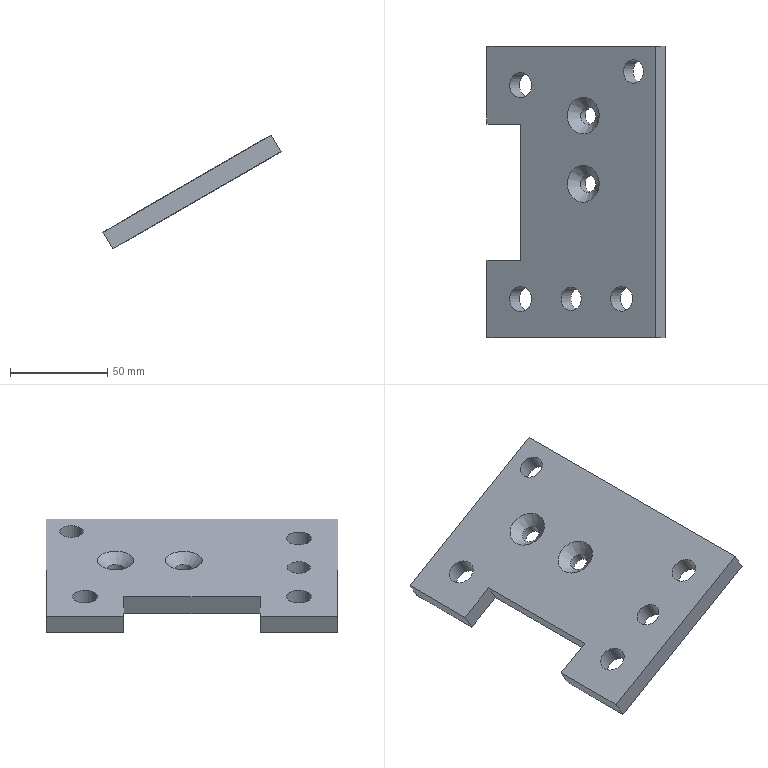Part | NX | features solid 2 | 1 solid | 19 faces | box 91.603 x 150 x 58.66 mm | volume 127515 mm3 | plane 10 | cylinder 7 | cone 2 | commonest cylinder face diameters 13 x3 9 x2 12 x2
STEP:
#1=CARTESIAN_POINT('',(89.575,759.782,201.044));
#2=VERTEX_POINT('',#1);
#3=CARTESIAN_POINT('',(89.575,764.282,201.044));
#4=DIRECTION('',(-0.5,0.,0.866));
#5=DIRECTION('',(0.,-1.,0.));
#6=AXIS2_PLACEMENT_3D('',#3,#4,#5);
#7=CIRCLE('',#6,4.5);
#8=EDGE_CURVE('',#2,#2,#7,.T.);
#9=ORIENTED_EDGE('',*,*,#8,.T.);
#10=EDGE_LOOP('',(#9));
#11=FACE_BOUND('',#10,.T.);
#12=CARTESIAN_POINT('',(120.538,787.,218.92));
#13=VERTEX_POINT('',#12);
#14=CARTESIAN_POINT('',(115.342,787.,215.92));
#15=DIRECTION('',(-0.5,0.,0.866));
#16=DIRECTION('',(0.866,0.,0.5));
#17=AXIS2_PLACEMENT_3D('',#14,#15,#16);
#18=CIRCLE('',#17,6.);
#19=EDGE_CURVE('',#13,#13,#18,.T.);
#20=ORIENTED_EDGE('',*,*,#19,.T.);
#21=EDGE_LOOP('',(#20));
#22=FACE_BOUND('',#21,.T.);
#23=CARTESIAN_POINT('',(62.947,670.,185.67));
#24=VERTEX_POINT('',#23);
#25=CARTESIAN_POINT('',(57.318,670.,182.42));
#26=DIRECTION('',(-0.5,0.,0.866));
#27=DIRECTION('',(0.866,0.,0.5));
#28=AXIS2_PLACEMENT_3D('',#25,#26,#27);
#29=CIRCLE('',#28,6.5);
#30=EDGE_CURVE('',#24,#24,#29,.T.);
#31=ORIENTED_EDGE('',*,*,#30,.T.);
#32=EDGE_LOOP('',(#31));
#33=FACE_BOUND('',#32,.T.);
#34=CARTESIAN_POINT('',(39.997,650.,172.42));
#35=VERTEX_POINT('',#34);
#36=CARTESIAN_POINT('',(39.997,690.,172.42));
#37=VERTEX_POINT('',#36);
#38=CARTESIAN_POINT('',(39.997,650.,172.42));
#39=DIRECTION('',(0.,-1.,0.));
#40=VECTOR('',#39,1000.);
#41=LINE('',#38,#40);
#42=EDGE_CURVE('',#35,#37,#41,.F.);
#43=ORIENTED_EDGE('',*,*,#42,.T.);
#44=CARTESIAN_POINT('',(57.318,690.,182.42));
#45=VERTEX_POINT('',#44);
#46=CARTESIAN_POINT('',(111.6,690.,213.759));
#47=DIRECTION('',(-0.866,0.,-0.5));
#48=VECTOR('',#47,1000.);
#49=LINE('',#46,#48);
#50=EDGE_CURVE('',#37,#45,#49,.F.);
#51=ORIENTED_EDGE('',*,*,#50,.T.);
#52=CARTESIAN_POINT('',(57.318,760.,182.42));
#53=VERTEX_POINT('',#52);
#54=CARTESIAN_POINT('',(57.318,650.,182.42));
#55=DIRECTION('',(0.,-1.,0.));
#56=VECTOR('',#55,1000.);
#57=LINE('',#54,#56);
#58=EDGE_CURVE('',#45,#53,#57,.F.);
#59=ORIENTED_EDGE('',*,*,#58,.T.);
#60=CARTESIAN_POINT('',(39.997,760.,172.42));
#61=VERTEX_POINT('',#60);
#62=CARTESIAN_POINT('',(24.997,760.,163.759));
#63=DIRECTION('',(0.866,0.,0.5));
#64=VECTOR('',#63,1000.);
#65=LINE('',#62,#64);
#66=EDGE_CURVE('',#61,#53,#65,.T.);
#67=ORIENTED_EDGE('',*,*,#66,.F.);
#68=CARTESIAN_POINT('',(39.997,800.,172.42));
#69=VERTEX_POINT('',#68);
#70=CARTESIAN_POINT('',(39.997,650.,172.42));
#71=DIRECTION('',(0.,-1.,0.));
#72=VECTOR('',#71,1000.);
#73=LINE('',#70,#72);
#74=EDGE_CURVE('',#61,#69,#73,.F.);
#75=ORIENTED_EDGE('',*,*,#74,.T.);
#76=CARTESIAN_POINT('',(126.6,800.,222.42));
#77=VERTEX_POINT('',#76);
#78=CARTESIAN_POINT('',(111.6,800.,213.759));
#79=DIRECTION('',(-0.866,0.,-0.5));
#80=VECTOR('',#79,1000.);
#81=LINE('',#78,#80);
#82=EDGE_CURVE('',#77,#69,#81,.T.);
#83=ORIENTED_EDGE('',*,*,#82,.F.);
#84=CARTESIAN_POINT('',(126.6,650.,222.42));
#85=VERTEX_POINT('',#84);
#86=CARTESIAN_POINT('',(126.6,650.,222.42));
#87=DIRECTION('',(0.,1.,0.));
#88=VECTOR('',#87,1000.);
#89=LINE('',#86,#88);
#90=EDGE_CURVE('',#85,#77,#89,.T.);
#91=ORIENTED_EDGE('',*,*,#90,.F.);
#92=CARTESIAN_POINT('',(111.6,650.,213.759));
#93=DIRECTION('',(0.866,0.,0.5));
#94=VECTOR('',#93,1000.);
#95=LINE('',#92,#94);
#96=EDGE_CURVE('',#85,#35,#95,.F.);
#97=ORIENTED_EDGE('',*,*,#96,.T.);
#98=EDGE_LOOP('',(#43,#51,#59,#67,#75,#83,#91,#97));
#99=FACE_BOUND('',#98,.T.);
#100=CARTESIAN_POINT('',(62.947,780.,185.67));
#101=VERTEX_POINT('',#100);
#102=CARTESIAN_POINT('',(57.318,780.,182.42));
#103=DIRECTION('',(-0.5,0.,0.866));
#104=DIRECTION('',(0.866,0.,0.5));
#105=AXIS2_PLACEMENT_3D('',#102,#103,#104);
#106=CIRCLE('',#105,6.5);
#107=EDGE_CURVE('',#101,#101,#106,.T.);
#108=ORIENTED_EDGE('',*,*,#107,.T.);
#109=EDGE_LOOP('',(#108));
#110=FACE_BOUND('',#109,.T.);
#111=CARTESIAN_POINT('',(114.909,670.,215.67));
#112=VERTEX_POINT('',#111);
#113=CARTESIAN_POINT('',(109.279,670.,212.42));
#114=DIRECTION('',(-0.5,0.,0.866));
#115=DIRECTION('',(0.866,0.,0.5));
#116=AXIS2_PLACEMENT_3D('',#113,#114,#115);
#117=CIRCLE('',#116,6.5);
#118=EDGE_CURVE('',#112,#112,#117,.T.);
#119=ORIENTED_EDGE('',*,*,#118,.T.);
#120=EDGE_LOOP('',(#119));
#121=FACE_BOUND('',#120,.T.);
#122=CARTESIAN_POINT('',(88.495,670.,200.42));
#123=VERTEX_POINT('',#122);
#124=CARTESIAN_POINT('',(83.299,670.,197.42));
#125=DIRECTION('',(-0.5,0.,0.866));
#126=DIRECTION('',(0.866,0.,0.5));
#127=AXIS2_PLACEMENT_3D('',#124,#125,#126);
#128=CIRCLE('',#127,6.);
#129=EDGE_CURVE('',#123,#123,#128,.T.);
#130=ORIENTED_EDGE('',*,*,#129,.T.);
#131=EDGE_LOOP('',(#130));
#132=FACE_BOUND('',#131,.T.);
#133=CARTESIAN_POINT('',(89.542,724.74,201.024));
#134=VERTEX_POINT('',#133);
#135=CARTESIAN_POINT('',(89.542,729.24,201.024));
#136=DIRECTION('',(-0.5,0.,0.866));
#137=DIRECTION('',(0.,-1.,0.));
#138=AXIS2_PLACEMENT_3D('',#135,#136,#137);
#139=CIRCLE('',#138,4.5);
#140=EDGE_CURVE('',#134,#134,#139,.T.);
#141=ORIENTED_EDGE('',*,*,#140,.T.);
#142=EDGE_LOOP('',(#141));
#143=FACE_BOUND('',#142,.T.);
#144=CARTESIAN_POINT('',(111.6,650.,213.759));
#145=DIRECTION('',(-0.5,0.,0.866));
#146=DIRECTION('',(-0.866,0.,-0.5));
#147=AXIS2_PLACEMENT_3D('',#144,#145,#146);
#148=PLANE('',#147);
#149=ADVANCED_FACE('',(#11,#22,#33,#99,#110,#121,#132,#143),#148,.F.);
#150=CARTESIAN_POINT('',(92.803,764.282,214.454));
#151=VERTEX_POINT('',#150);
#152=CARTESIAN_POINT('',(84.575,764.282,209.704));
#153=DIRECTION('',(-0.5,0.,0.866));
#154=DIRECTION('',(0.866,0.,0.5));
#155=AXIS2_PLACEMENT_3D('',#152,#153,#154);
#156=CIRCLE('',#155,9.5);
#157=EDGE_CURVE('',#151,#151,#156,.T.);
#158=ORIENTED_EDGE('',*,*,#157,.F.);
#159=EDGE_LOOP('',(#158));
#160=FACE_BOUND('',#159,.T.);
#161=CARTESIAN_POINT('',(92.769,729.24,214.434));
#162=VERTEX_POINT('',#161);
#163=CARTESIAN_POINT('',(84.542,729.24,209.684));
#164=DIRECTION('',(-0.5,0.,0.866));
#165=DIRECTION('',(0.866,0.,0.5));
#166=AXIS2_PLACEMENT_3D('',#163,#164,#165);
#167=CIRCLE('',#166,9.5);
#168=EDGE_CURVE('',#162,#162,#167,.T.);
#169=ORIENTED_EDGE('',*,*,#168,.F.);
#170=EDGE_LOOP('',(#169));
#171=FACE_BOUND('',#170,.T.);
#172=CARTESIAN_POINT('',(115.538,787.,227.58));
#173=VERTEX_POINT('',#172);
#174=CARTESIAN_POINT('',(110.342,787.,224.58));
#175=DIRECTION('',(-0.5,0.,0.866));
#176=DIRECTION('',(0.866,0.,0.5));
#177=AXIS2_PLACEMENT_3D('',#174,#175,#176);
#178=CIRCLE('',#177,6.);
#179=EDGE_CURVE('',#173,#173,#178,.T.);
#180=ORIENTED_EDGE('',*,*,#179,.F.);
#181=EDGE_LOOP('',(#180));
#182=FACE_BOUND('',#181,.T.);
#183=CARTESIAN_POINT('',(57.947,670.,194.33));
#184=VERTEX_POINT('',#183);
#185=CARTESIAN_POINT('',(52.318,670.,191.08));
#186=DIRECTION('',(-0.5,0.,0.866));
#187=DIRECTION('',(0.866,0.,0.5));
#188=AXIS2_PLACEMENT_3D('',#185,#186,#187);
#189=CIRCLE('',#188,6.5);
#190=EDGE_CURVE('',#184,#184,#189,.T.);
#191=ORIENTED_EDGE('',*,*,#190,.F.);
#192=EDGE_LOOP('',(#191));
#193=FACE_BOUND('',#192,.T.);
#194=CARTESIAN_POINT('',(34.997,690.,181.08));
#195=VERTEX_POINT('',#194);
#196=CARTESIAN_POINT('',(52.318,690.,191.08));
#197=VERTEX_POINT('',#196);
#198=CARTESIAN_POINT('',(19.997,690.,172.42));
#199=DIRECTION('',(-0.866,0.,-0.5));
#200=VECTOR('',#199,1000.);
#201=LINE('',#198,#200);
#202=EDGE_CURVE('',#195,#197,#201,.F.);
#203=ORIENTED_EDGE('',*,*,#202,.F.);
#204=CARTESIAN_POINT('',(34.997,650.,181.08));
#205=VERTEX_POINT('',#204);
#206=CARTESIAN_POINT('',(34.997,650.,181.08));
#207=DIRECTION('',(0.,-1.,0.));
#208=VECTOR('',#207,1000.);
#209=LINE('',#206,#208);
#210=EDGE_CURVE('',#205,#195,#209,.F.);
#211=ORIENTED_EDGE('',*,*,#210,.F.);
#212=CARTESIAN_POINT('',(121.6,650.,231.08));
#213=VERTEX_POINT('',#212);
#214=CARTESIAN_POINT('',(106.6,650.,222.42));
#215=DIRECTION('',(-0.866,0.,-0.5));
#216=VECTOR('',#215,1000.);
#217=LINE('',#214,#216);
#218=EDGE_CURVE('',#213,#205,#217,.T.);
#219=ORIENTED_EDGE('',*,*,#218,.F.);
#220=CARTESIAN_POINT('',(121.6,800.,231.08));
#221=VERTEX_POINT('',#220);
#222=CARTESIAN_POINT('',(121.6,650.,231.08));
#223=DIRECTION('',(0.,1.,0.));
#224=VECTOR('',#223,1000.);
#225=LINE('',#222,#224);
#226=EDGE_CURVE('',#213,#221,#225,.T.);
#227=ORIENTED_EDGE('',*,*,#226,.T.);
#228=CARTESIAN_POINT('',(34.997,800.,181.08));
#229=VERTEX_POINT('',#228);
#230=CARTESIAN_POINT('',(106.6,800.,222.42));
#231=DIRECTION('',(-0.866,0.,-0.5));
#232=VECTOR('',#231,1000.);
#233=LINE('',#230,#232);
#234=EDGE_CURVE('',#221,#229,#233,.T.);
#235=ORIENTED_EDGE('',*,*,#234,.T.);
#236=CARTESIAN_POINT('',(34.997,760.,181.08));
#237=VERTEX_POINT('',#236);
#238=CARTESIAN_POINT('',(34.997,650.,181.08));
#239=DIRECTION('',(0.,-1.,0.));
#240=VECTOR('',#239,1000.);
#241=LINE('',#238,#240);
#242=EDGE_CURVE('',#237,#229,#241,.F.);
#243=ORIENTED_EDGE('',*,*,#242,.F.);
#244=CARTESIAN_POINT('',(52.318,760.,191.08));
#245=VERTEX_POINT('',#244);
#246=CARTESIAN_POINT('',(19.997,760.,172.42));
#247=DIRECTION('',(0.866,0.,0.5));
#248=VECTOR('',#247,1000.);
#249=LINE('',#246,#248);
#250=EDGE_CURVE('',#237,#245,#249,.T.);
#251=ORIENTED_EDGE('',*,*,#250,.T.);
#252=CARTESIAN_POINT('',(52.318,650.,191.08));
#253=DIRECTION('',(0.,-1.,0.));
#254=VECTOR('',#253,1000.);
#255=LINE('',#252,#254);
#256=EDGE_CURVE('',#197,#245,#255,.F.);
#257=ORIENTED_EDGE('',*,*,#256,.F.);
#258=EDGE_LOOP('',(#203,#211,#219,#227,#235,#243,#251,#257));
#259=FACE_BOUND('',#258,.T.);
#260=CARTESIAN_POINT('',(57.947,780.,194.33));
#261=VERTEX_POINT('',#260);
#262=CARTESIAN_POINT('',(52.318,780.,191.08));
#263=DIRECTION('',(-0.5,0.,0.866));
#264=DIRECTION('',(0.866,0.,0.5));
#265=AXIS2_PLACEMENT_3D('',#262,#263,#264);
#266=CIRCLE('',#265,6.5);
#267=EDGE_CURVE('',#261,#261,#266,.T.);
#268=ORIENTED_EDGE('',*,*,#267,.F.);
#269=EDGE_LOOP('',(#268));
#270=FACE_BOUND('',#269,.T.);
#271=CARTESIAN_POINT('',(109.909,670.,224.33));
#272=VERTEX_POINT('',#271);
#273=CARTESIAN_POINT('',(104.279,670.,221.08));
#274=DIRECTION('',(-0.5,0.,0.866));
#275=DIRECTION('',(0.866,0.,0.5));
#276=AXIS2_PLACEMENT_3D('',#273,#274,#275);
#277=CIRCLE('',#276,6.5);
#278=EDGE_CURVE('',#272,#272,#277,.T.);
#279=ORIENTED_EDGE('',*,*,#278,.F.);
#280=EDGE_LOOP('',(#279));
#281=FACE_BOUND('',#280,.T.);
#282=CARTESIAN_POINT('',(83.495,670.,209.08));
#283=VERTEX_POINT('',#282);
#284=CARTESIAN_POINT('',(78.299,670.,206.08));
#285=DIRECTION('',(-0.5,0.,0.866));
#286=DIRECTION('',(0.866,0.,0.5));
#287=AXIS2_PLACEMENT_3D('',#284,#285,#286);
#288=CIRCLE('',#287,6.);
#289=EDGE_CURVE('',#283,#283,#288,.T.);
#290=ORIENTED_EDGE('',*,*,#289,.F.);
#291=EDGE_LOOP('',(#290));
#292=FACE_BOUND('',#291,.T.);
#293=CARTESIAN_POINT('',(106.6,650.,222.42));
#294=DIRECTION('',(-0.5,0.,0.866));
#295=DIRECTION('',(-0.866,0.,-0.5));
#296=AXIS2_PLACEMENT_3D('',#293,#294,#295);
#297=PLANE('',#296);
#298=ADVANCED_FACE('',(#160,#171,#182,#193,#259,#270,#281,#292),#297,.T.);
#299=CARTESIAN_POINT('',(34.997,690.,181.08));
#300=DIRECTION('',(-0.5,0.,0.866));
#301=VECTOR('',#300,1000.);
#302=LINE('',#299,#301);
#303=EDGE_CURVE('',#37,#195,#302,.T.);
#304=ORIENTED_EDGE('',*,*,#303,.F.);
#305=ORIENTED_EDGE('',*,*,#42,.F.);
#306=CARTESIAN_POINT('',(34.997,650.,181.08));
#307=DIRECTION('',(0.5,0.,-0.866));
#308=VECTOR('',#307,1000.);
#309=LINE('',#306,#308);
#310=EDGE_CURVE('',#205,#35,#309,.T.);
#311=ORIENTED_EDGE('',*,*,#310,.F.);
#312=ORIENTED_EDGE('',*,*,#210,.T.);
#313=EDGE_LOOP('',(#304,#305,#311,#312));
#314=FACE_BOUND('',#313,.T.);
#315=CARTESIAN_POINT('',(34.997,650.,181.08));
#316=DIRECTION('',(0.866,0.,0.5));
#317=DIRECTION('',(0.,1.,0.));
#318=AXIS2_PLACEMENT_3D('',#315,#316,#317);
#319=PLANE('',#318);
#320=ADVANCED_FACE('',(#314),#319,.F.);
#321=CARTESIAN_POINT('',(121.6,800.,231.08));
#322=DIRECTION('',(0.5,0.,-0.866));
#323=VECTOR('',#322,1000.);
#324=LINE('',#321,#323);
#325=EDGE_CURVE('',#221,#77,#324,.T.);
#326=ORIENTED_EDGE('',*,*,#325,.F.);
#327=ORIENTED_EDGE('',*,*,#226,.F.);
#328=CARTESIAN_POINT('',(121.6,650.,231.08));
#329=DIRECTION('',(-0.5,0.,0.866));
#330=VECTOR('',#329,1000.);
#331=LINE('',#328,#330);
#332=EDGE_CURVE('',#213,#85,#331,.F.);
#333=ORIENTED_EDGE('',*,*,#332,.T.);
#334=ORIENTED_EDGE('',*,*,#90,.T.);
#335=EDGE_LOOP('',(#326,#327,#333,#334));
#336=FACE_BOUND('',#335,.T.);
#337=CARTESIAN_POINT('',(121.6,650.,231.08));
#338=DIRECTION('',(0.866,0.,0.5));
#339=DIRECTION('',(0.,1.,0.));
#340=AXIS2_PLACEMENT_3D('',#337,#338,#339);
#341=PLANE('',#340);
#342=ADVANCED_FACE('',(#336),#341,.T.);
#343=ORIENTED_EDGE('',*,*,#332,.F.);
#344=ORIENTED_EDGE('',*,*,#218,.T.);
#345=ORIENTED_EDGE('',*,*,#310,.T.);
#346=ORIENTED_EDGE('',*,*,#96,.F.);
#347=EDGE_LOOP('',(#343,#344,#345,#346));
#348=FACE_BOUND('',#347,.T.);
#349=CARTESIAN_POINT('',(106.6,650.,222.42));
#350=DIRECTION('',(0.,1.,0.));
#351=DIRECTION('',(-0.866,0.,-0.5));
#352=AXIS2_PLACEMENT_3D('',#349,#350,#351);
#353=PLANE('',#352);
#354=ADVANCED_FACE('',(#348),#353,.F.);
#355=CARTESIAN_POINT('',(37.497,760.,176.75));
#356=DIRECTION('',(0.5,0.,-0.866));
#357=VECTOR('',#356,1000.);
#358=LINE('',#355,#357);
#359=EDGE_CURVE('',#61,#237,#358,.F.);
#360=ORIENTED_EDGE('',*,*,#359,.T.);
#361=ORIENTED_EDGE('',*,*,#242,.T.);
#362=CARTESIAN_POINT('',(34.997,800.,181.08));
#363=DIRECTION('',(-0.5,0.,0.866));
#364=VECTOR('',#363,1000.);
#365=LINE('',#362,#364);
#366=EDGE_CURVE('',#229,#69,#365,.F.);
#367=ORIENTED_EDGE('',*,*,#366,.T.);
#368=ORIENTED_EDGE('',*,*,#74,.F.);
#369=EDGE_LOOP('',(#360,#361,#367,#368));
#370=FACE_BOUND('',#369,.T.);
#371=CARTESIAN_POINT('',(34.997,650.,181.08));
#372=DIRECTION('',(0.866,0.,0.5));
#373=DIRECTION('',(0.,1.,0.));
#374=AXIS2_PLACEMENT_3D('',#371,#372,#373);
#375=PLANE('',#374);
#376=ADVANCED_FACE('',(#370),#375,.F.);
#377=ORIENTED_EDGE('',*,*,#234,.F.);
#378=ORIENTED_EDGE('',*,*,#325,.T.);
#379=ORIENTED_EDGE('',*,*,#82,.T.);
#380=ORIENTED_EDGE('',*,*,#366,.F.);
#381=EDGE_LOOP('',(#377,#378,#379,#380));
#382=FACE_BOUND('',#381,.T.);
#383=CARTESIAN_POINT('',(106.6,800.,222.42));
#384=DIRECTION('',(0.,1.,0.));
#385=DIRECTION('',(-0.866,0.,-0.5));
#386=AXIS2_PLACEMENT_3D('',#383,#384,#385);
#387=PLANE('',#386);
#388=ADVANCED_FACE('',(#382),#387,.T.);
#389=ORIENTED_EDGE('',*,*,#303,.T.);
#390=ORIENTED_EDGE('',*,*,#202,.T.);
#391=CARTESIAN_POINT('',(54.818,690.,186.75));
#392=DIRECTION('',(-0.5,0.,0.866));
#393=VECTOR('',#392,1000.);
#394=LINE('',#391,#393);
#395=EDGE_CURVE('',#45,#197,#394,.T.);
#396=ORIENTED_EDGE('',*,*,#395,.F.);
#397=ORIENTED_EDGE('',*,*,#50,.F.);
#398=EDGE_LOOP('',(#389,#390,#396,#397));
#399=FACE_BOUND('',#398,.T.);
#400=CARTESIAN_POINT('',(22.497,690.,168.09));
#401=DIRECTION('',(0.,1.,0.));
#402=DIRECTION('',(0.866,0.,0.5));
#403=AXIS2_PLACEMENT_3D('',#400,#401,#402);
#404=PLANE('',#403);
#405=ADVANCED_FACE('',(#399),#404,.T.);
#406=ORIENTED_EDGE('',*,*,#395,.T.);
#407=ORIENTED_EDGE('',*,*,#256,.T.);
#408=CARTESIAN_POINT('',(54.818,760.,186.75));
#409=DIRECTION('',(0.5,0.,-0.866));
#410=VECTOR('',#409,1000.);
#411=LINE('',#408,#410);
#412=EDGE_CURVE('',#53,#245,#411,.F.);
#413=ORIENTED_EDGE('',*,*,#412,.F.);
#414=ORIENTED_EDGE('',*,*,#58,.F.);
#415=EDGE_LOOP('',(#406,#407,#413,#414));
#416=FACE_BOUND('',#415,.T.);
#417=CARTESIAN_POINT('',(54.818,650.,186.75));
#418=DIRECTION('',(-0.866,0.,-0.5));
#419=DIRECTION('',(0.,1.,0.));
#420=AXIS2_PLACEMENT_3D('',#417,#418,#419);
#421=PLANE('',#420);
#422=ADVANCED_FACE('',(#416),#421,.T.);
#423=ORIENTED_EDGE('',*,*,#66,.T.);
#424=ORIENTED_EDGE('',*,*,#412,.T.);
#425=ORIENTED_EDGE('',*,*,#250,.F.);
#426=ORIENTED_EDGE('',*,*,#359,.F.);
#427=EDGE_LOOP('',(#423,#424,#425,#426));
#428=FACE_BOUND('',#427,.T.);
#429=CARTESIAN_POINT('',(22.497,760.,168.09));
#430=DIRECTION('',(0.,1.,0.));
#431=DIRECTION('',(0.866,0.,0.5));
#432=AXIS2_PLACEMENT_3D('',#429,#430,#431);
#433=PLANE('',#432);
#434=ADVANCED_FACE('',(#428),#433,.F.);
#435=ORIENTED_EDGE('',*,*,#267,.T.);
#436=EDGE_LOOP('',(#435));
#437=FACE_BOUND('',#436,.T.);
#438=ORIENTED_EDGE('',*,*,#107,.F.);
#439=EDGE_LOOP('',(#438));
#440=FACE_BOUND('',#439,.T.);
#441=CARTESIAN_POINT('',(52.318,780.,191.08));
#442=DIRECTION('',(0.5,0.,-0.866));
#443=DIRECTION('',(-0.866,0.,-0.5));
#444=AXIS2_PLACEMENT_3D('',#441,#442,#443);
#445=CYLINDRICAL_SURFACE('',#444,6.5);
#446=ADVANCED_FACE('',(#437,#440),#445,.F.);
#447=ORIENTED_EDGE('',*,*,#190,.T.);
#448=EDGE_LOOP('',(#447));
#449=FACE_BOUND('',#448,.T.);
#450=ORIENTED_EDGE('',*,*,#30,.F.);
#451=EDGE_LOOP('',(#450));
#452=FACE_BOUND('',#451,.T.);
#453=CARTESIAN_POINT('',(52.318,670.,191.08));
#454=DIRECTION('',(0.5,0.,-0.866));
#455=DIRECTION('',(-0.866,0.,-0.5));
#456=AXIS2_PLACEMENT_3D('',#453,#454,#455);
#457=CYLINDRICAL_SURFACE('',#456,6.5);
#458=ADVANCED_FACE('',(#449,#452),#457,.F.);
#459=ORIENTED_EDGE('',*,*,#278,.T.);
#460=EDGE_LOOP('',(#459));
#461=FACE_BOUND('',#460,.T.);
#462=ORIENTED_EDGE('',*,*,#118,.F.);
#463=EDGE_LOOP('',(#462));
#464=FACE_BOUND('',#463,.T.);
#465=CARTESIAN_POINT('',(104.279,670.,221.08));
#466=DIRECTION('',(0.5,0.,-0.866));
#467=DIRECTION('',(-0.866,0.,-0.5));
#468=AXIS2_PLACEMENT_3D('',#465,#466,#467);
#469=CYLINDRICAL_SURFACE('',#468,6.5);
#470=ADVANCED_FACE('',(#461,#464),#469,.F.);
#471=ORIENTED_EDGE('',*,*,#179,.T.);
#472=EDGE_LOOP('',(#471));
#473=FACE_BOUND('',#472,.T.);
#474=ORIENTED_EDGE('',*,*,#19,.F.);
#475=EDGE_LOOP('',(#474));
#476=FACE_BOUND('',#475,.T.);
#477=CARTESIAN_POINT('',(110.342,787.,224.58));
#478=DIRECTION('',(0.5,0.,-0.866));
#479=DIRECTION('',(-0.866,0.,-0.5));
#480=AXIS2_PLACEMENT_3D('',#477,#478,#479);
#481=CYLINDRICAL_SURFACE('',#480,6.);
#482=ADVANCED_FACE('',(#473,#476),#481,.F.);
#483=ORIENTED_EDGE('',*,*,#289,.T.);
#484=EDGE_LOOP('',(#483));
#485=FACE_BOUND('',#484,.T.);
#486=ORIENTED_EDGE('',*,*,#129,.F.);
#487=EDGE_LOOP('',(#486));
#488=FACE_BOUND('',#487,.T.);
#489=CARTESIAN_POINT('',(78.299,670.,206.08));
#490=DIRECTION('',(0.5,0.,-0.866));
#491=DIRECTION('',(-0.866,0.,-0.5));
#492=AXIS2_PLACEMENT_3D('',#489,#490,#491);
#493=CYLINDRICAL_SURFACE('',#492,6.);
#494=ADVANCED_FACE('',(#485,#488),#493,.F.);
#495=CARTESIAN_POINT('',(90.973,764.282,207.624));
#496=VERTEX_POINT('',#495);
#497=CARTESIAN_POINT('',(87.075,764.282,205.374));
#498=DIRECTION('',(-0.5,0.,0.866));
#499=DIRECTION('',(0.866,0.,0.5));
#500=AXIS2_PLACEMENT_3D('',#497,#498,#499);
#501=CIRCLE('',#500,4.5);
#502=EDGE_CURVE('',#496,#496,#501,.F.);
#503=ORIENTED_EDGE('',*,*,#502,.F.);
#504=EDGE_LOOP('',(#503));
#505=FACE_BOUND('',#504,.T.);
#506=ORIENTED_EDGE('',*,*,#8,.F.);
#507=EDGE_LOOP('',(#506));
#508=FACE_BOUND('',#507,.T.);
#509=CARTESIAN_POINT('',(87.075,764.282,205.374));
#510=DIRECTION('',(0.5,0.,-0.866));
#511=DIRECTION('',(-0.866,0.,-0.5));
#512=AXIS2_PLACEMENT_3D('',#509,#510,#511);
#513=CYLINDRICAL_SURFACE('',#512,4.5);
#514=ADVANCED_FACE('',(#505,#508),#513,.F.);
#515=CARTESIAN_POINT('',(87.042,724.74,205.354));
#516=VERTEX_POINT('',#515);
#517=CARTESIAN_POINT('',(87.042,729.24,205.354));
#518=DIRECTION('',(-0.5,0.,0.866));
#519=DIRECTION('',(0.,-1.,0.));
#520=AXIS2_PLACEMENT_3D('',#517,#518,#519);
#521=CIRCLE('',#520,4.5);
#522=EDGE_CURVE('',#516,#516,#521,.T.);
#523=ORIENTED_EDGE('',*,*,#522,.F.);
#524=EDGE_LOOP('',(#523));
#525=FACE_BOUND('',#524,.T.);
#526=ORIENTED_EDGE('',*,*,#168,.T.);
#527=EDGE_LOOP('',(#526));
#528=FACE_BOUND('',#527,.T.);
#529=CARTESIAN_POINT('',(84.542,729.24,209.684));
#530=DIRECTION('',(-0.5,0.,0.866));
#531=DIRECTION('',(0.866,0.,0.5));
#532=AXIS2_PLACEMENT_3D('',#529,#530,#531);
#533=CONICAL_SURFACE('',#532,9.5,0.7854);
#534=ADVANCED_FACE('',(#525,#528),#533,.F.);
#535=ORIENTED_EDGE('',*,*,#522,.T.);
#536=EDGE_LOOP('',(#535));
#537=FACE_BOUND('',#536,.T.);
#538=ORIENTED_EDGE('',*,*,#140,.F.);
#539=EDGE_LOOP('',(#538));
#540=FACE_BOUND('',#539,.T.);
#541=CARTESIAN_POINT('',(87.042,729.24,205.354));
#542=DIRECTION('',(0.5,0.,-0.866));
#543=DIRECTION('',(-0.866,0.,-0.5));
#544=AXIS2_PLACEMENT_3D('',#541,#542,#543);
#545=CYLINDRICAL_SURFACE('',#544,4.5);
#546=ADVANCED_FACE('',(#537,#540),#545,.F.);
#547=ORIENTED_EDGE('',*,*,#502,.T.);
#548=EDGE_LOOP('',(#547));
#549=FACE_BOUND('',#548,.T.);
#550=ORIENTED_EDGE('',*,*,#157,.T.);
#551=EDGE_LOOP('',(#550));
#552=FACE_BOUND('',#551,.T.);
#553=CARTESIAN_POINT('',(84.575,764.282,209.704));
#554=DIRECTION('',(-0.5,0.,0.866));
#555=DIRECTION('',(0.866,0.,0.5));
#556=AXIS2_PLACEMENT_3D('',#553,#554,#555);
#557=CONICAL_SURFACE('',#556,9.5,0.7854);
#558=ADVANCED_FACE('',(#549,#552),#557,.F.);
#559=CLOSED_SHELL('',(#149,#298,#320,#342,#354,#376,#388,#405,#422,#434,#446,#458,#470,#482,#494,#514,#534,#546,#558));
#560=MANIFOLD_SOLID_BREP('',#559);
#561=(LENGTH_UNIT()NAMED_UNIT(*)SI_UNIT(.MILLI.,.METRE.));
#562=UNCERTAINTY_MEASURE_WITH_UNIT(LENGTH_MEASURE(0.00001),#561,'','');
#563=(NAMED_UNIT(*)PLANE_ANGLE_UNIT()SI_UNIT($,.RADIAN.));
#564=(NAMED_UNIT(*)SI_UNIT($,.STERADIAN.)SOLID_ANGLE_UNIT());
#565=(GEOMETRIC_REPRESENTATION_CONTEXT(3)GLOBAL_UNCERTAINTY_ASSIGNED_CONTEXT((#562))GLOBAL_UNIT_ASSIGNED_CONTEXT((#561,#563,#564))REPRESENTATION_CONTEXT('',''));
#566=ADVANCED_BREP_SHAPE_REPRESENTATION('',(#560),#565);